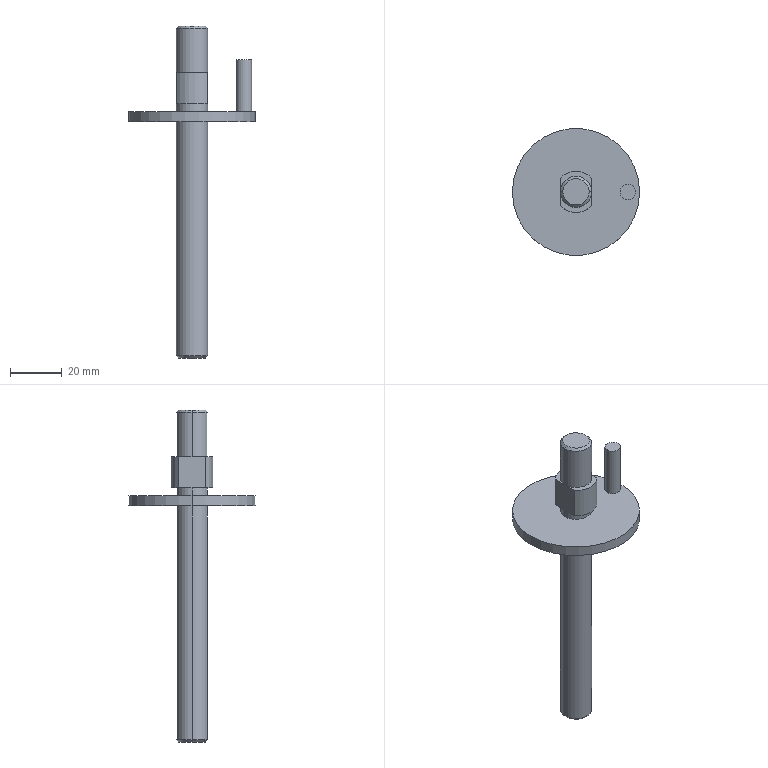Part | SolidWorks | features ICE 5, Chamfer 1, Extrusion 1 | 1 solid | 27 faces | box 49 x 49 x 128 mm | volume 22811 mm3 | cylinder 12 | plane 11 | cone 4 | commonest cylinder face diameters 12 x6 6 x2 16 x2 49 x2
STEP:
#1=CARTESIAN_POINT('',(23.,0.,115.));
#2=VERTEX_POINT('',#1);
#3=CARTESIAN_POINT('',(17.,0.,115.));
#4=VERTEX_POINT('',#3);
#5=CARTESIAN_POINT('',(20.,0.,115.));
#6=DIRECTION('',(0.,0.,1.));
#7=DIRECTION('',(1.,0.,0.));
#8=AXIS2_PLACEMENT_3D('',#5,#6,#7);
#9=CIRCLE('',#8,3.);
#10=EDGE_CURVE('',#2,#4,#9,.T.);
#11=ORIENTED_EDGE('',*,*,#10,.F.);
#12=CARTESIAN_POINT('',(23.,0.,95.));
#13=VERTEX_POINT('',#12);
#14=CARTESIAN_POINT('',(23.,0.,115.));
#15=DIRECTION('',(0.,0.,-1.));
#16=VECTOR('',#15,1000.);
#17=LINE('',#14,#16);
#18=EDGE_CURVE('',#2,#13,#17,.T.);
#19=ORIENTED_EDGE('',*,*,#18,.T.);
#20=CARTESIAN_POINT('',(17.,0.,95.));
#21=VERTEX_POINT('',#20);
#22=CARTESIAN_POINT('',(20.,0.,95.));
#23=DIRECTION('',(0.,0.,1.));
#24=DIRECTION('',(1.,0.,0.));
#25=AXIS2_PLACEMENT_3D('',#22,#23,#24);
#26=CIRCLE('',#25,3.);
#27=EDGE_CURVE('',#13,#21,#26,.T.);
#28=ORIENTED_EDGE('',*,*,#27,.T.);
#29=CARTESIAN_POINT('',(17.,0.,115.));
#30=DIRECTION('',(0.,0.,-1.));
#31=VECTOR('',#30,1000.);
#32=LINE('',#29,#31);
#33=EDGE_CURVE('',#4,#21,#32,.T.);
#34=ORIENTED_EDGE('',*,*,#33,.F.);
#35=EDGE_LOOP('',(#11,#19,#28,#34));
#36=FACE_OUTER_BOUND('',#35,.T.);
#37=CARTESIAN_POINT('',(20.,0.,115.));
#38=DIRECTION('',(0.,0.,-1.));
#39=DIRECTION('',(-1.,0.,0.));
#40=AXIS2_PLACEMENT_3D('',#37,#38,#39);
#41=CYLINDRICAL_SURFACE('',#40,3.);
#42=ADVANCED_FACE('',(#36),#41,.T.);
#43=CARTESIAN_POINT('',(5.1,0.,128.));
#44=VERTEX_POINT('',#43);
#45=CARTESIAN_POINT('',(-5.1,0.,128.));
#46=VERTEX_POINT('',#45);
#47=CARTESIAN_POINT('',(0.,0.,128.));
#48=DIRECTION('',(0.,0.,1.));
#49=DIRECTION('',(1.,0.,0.));
#50=AXIS2_PLACEMENT_3D('',#47,#48,#49);
#51=CIRCLE('',#50,5.1);
#52=EDGE_CURVE('',#44,#46,#51,.T.);
#53=ORIENTED_EDGE('',*,*,#52,.F.);
#54=CARTESIAN_POINT('',(6.,0.,127.1));
#55=VERTEX_POINT('',#54);
#56=CARTESIAN_POINT('',(5.1,0.,128.));
#57=DIRECTION('',(0.7071,0.,-0.7071));
#58=VECTOR('',#57,1000.);
#59=LINE('',#56,#58);
#60=EDGE_CURVE('',#44,#55,#59,.T.);
#61=ORIENTED_EDGE('',*,*,#60,.T.);
#62=CARTESIAN_POINT('',(-6.,0.,127.1));
#63=VERTEX_POINT('',#62);
#64=CARTESIAN_POINT('',(0.,0.,127.1));
#65=DIRECTION('',(0.,0.,-1.));
#66=DIRECTION('',(1.,0.,0.));
#67=AXIS2_PLACEMENT_3D('',#64,#65,#66);
#68=CIRCLE('',#67,6.);
#69=EDGE_CURVE('',#63,#55,#68,.T.);
#70=ORIENTED_EDGE('',*,*,#69,.F.);
#71=CARTESIAN_POINT('',(-5.1,0.,128.));
#72=DIRECTION('',(-0.7071,0.,-0.7071));
#73=VECTOR('',#72,1000.);
#74=LINE('',#71,#73);
#75=EDGE_CURVE('',#46,#63,#74,.T.);
#76=ORIENTED_EDGE('',*,*,#75,.F.);
#77=EDGE_LOOP('',(#53,#61,#70,#76));
#78=FACE_OUTER_BOUND('',#77,.T.);
#79=CARTESIAN_POINT('',(0.,0.,128.));
#80=DIRECTION('',(0.,0.,-1.));
#81=DIRECTION('',(-1.,0.,0.));
#82=AXIS2_PLACEMENT_3D('',#79,#80,#81);
#83=CONICAL_SURFACE('',#82,5.1,0.7854);
#84=ADVANCED_FACE('',(#78),#83,.T.);
#85=CARTESIAN_POINT('',(-5.1,0.,0.));
#86=VERTEX_POINT('',#85);
#87=CARTESIAN_POINT('',(5.1,0.,0.));
#88=VERTEX_POINT('',#87);
#89=CARTESIAN_POINT('',(0.,0.,0.));
#90=DIRECTION('',(0.,0.,-1.));
#91=DIRECTION('',(1.,0.,0.));
#92=AXIS2_PLACEMENT_3D('',#89,#90,#91);
#93=CIRCLE('',#92,5.1);
#94=EDGE_CURVE('',#86,#88,#93,.T.);
#95=ORIENTED_EDGE('',*,*,#94,.F.);
#96=CARTESIAN_POINT('',(-6.,0.,0.9));
#97=VERTEX_POINT('',#96);
#98=CARTESIAN_POINT('',(-6.,0.,0.9));
#99=DIRECTION('',(-0.7071,0.,0.7071));
#100=VECTOR('',#99,1000.);
#101=LINE('',#98,#100);
#102=EDGE_CURVE('',#86,#97,#101,.T.);
#103=ORIENTED_EDGE('',*,*,#102,.T.);
#104=CARTESIAN_POINT('',(6.,0.,0.9));
#105=VERTEX_POINT('',#104);
#106=CARTESIAN_POINT('',(0.,0.,0.9));
#107=DIRECTION('',(0.,0.,1.));
#108=DIRECTION('',(1.,0.,0.));
#109=AXIS2_PLACEMENT_3D('',#106,#107,#108);
#110=CIRCLE('',#109,6.);
#111=EDGE_CURVE('',#105,#97,#110,.T.);
#112=ORIENTED_EDGE('',*,*,#111,.F.);
#113=CARTESIAN_POINT('',(6.,0.,0.9));
#114=DIRECTION('',(0.7071,0.,0.7071));
#115=VECTOR('',#114,1000.);
#116=LINE('',#113,#115);
#117=EDGE_CURVE('',#88,#105,#116,.T.);
#118=ORIENTED_EDGE('',*,*,#117,.F.);
#119=EDGE_LOOP('',(#95,#103,#112,#118));
#120=FACE_OUTER_BOUND('',#119,.T.);
#121=CARTESIAN_POINT('',(0.,0.,0.9));
#122=DIRECTION('',(0.,0.,1.));
#123=DIRECTION('',(1.,0.,0.));
#124=AXIS2_PLACEMENT_3D('',#121,#122,#123);
#125=CONICAL_SURFACE('',#124,6.,0.7854);
#126=ADVANCED_FACE('',(#120),#125,.T.);
#127=ORIENTED_EDGE('',*,*,#69,.T.);
#128=CARTESIAN_POINT('',(6.,0.,110.));
#129=VERTEX_POINT('',#128);
#130=CARTESIAN_POINT('',(6.,0.,128.));
#131=DIRECTION('',(0.,0.,-1.));
#132=VECTOR('',#131,1000.);
#133=LINE('',#130,#132);
#134=EDGE_CURVE('',#55,#129,#133,.T.);
#135=ORIENTED_EDGE('',*,*,#134,.T.);
#136=CARTESIAN_POINT('',(-6.,0.,110.));
#137=VERTEX_POINT('',#136);
#138=CARTESIAN_POINT('',(0.,0.,110.));
#139=DIRECTION('',(0.,0.,1.));
#140=DIRECTION('',(1.,0.,0.));
#141=AXIS2_PLACEMENT_3D('',#138,#139,#140);
#142=CIRCLE('',#141,6.);
#143=EDGE_CURVE('',#129,#137,#142,.T.);
#144=ORIENTED_EDGE('',*,*,#143,.T.);
#145=CARTESIAN_POINT('',(-6.,0.,128.));
#146=DIRECTION('',(0.,0.,-1.));
#147=VECTOR('',#146,1000.);
#148=LINE('',#145,#147);
#149=EDGE_CURVE('',#63,#137,#148,.T.);
#150=ORIENTED_EDGE('',*,*,#149,.F.);
#151=EDGE_LOOP('',(#127,#135,#144,#150));
#152=FACE_OUTER_BOUND('',#151,.T.);
#153=CARTESIAN_POINT('',(0.,0.,128.));
#154=DIRECTION('',(0.,0.,-1.));
#155=DIRECTION('',(-1.,0.,0.));
#156=AXIS2_PLACEMENT_3D('',#153,#154,#155);
#157=CYLINDRICAL_SURFACE('',#156,6.);
#158=ADVANCED_FACE('',(#152),#157,.T.);
#159=CARTESIAN_POINT('',(6.,0.,98.));
#160=VERTEX_POINT('',#159);
#161=CARTESIAN_POINT('',(-6.,0.,98.));
#162=VERTEX_POINT('',#161);
#163=CARTESIAN_POINT('',(0.,0.,98.));
#164=DIRECTION('',(0.,0.,1.));
#165=DIRECTION('',(1.,0.,0.));
#166=AXIS2_PLACEMENT_3D('',#163,#164,#165);
#167=CIRCLE('',#166,6.);
#168=EDGE_CURVE('',#160,#162,#167,.T.);
#169=ORIENTED_EDGE('',*,*,#168,.F.);
#170=CARTESIAN_POINT('',(6.,0.,95.));
#171=VERTEX_POINT('',#170);
#172=CARTESIAN_POINT('',(6.,0.,98.));
#173=DIRECTION('',(0.,0.,-1.));
#174=VECTOR('',#173,1000.);
#175=LINE('',#172,#174);
#176=EDGE_CURVE('',#160,#171,#175,.T.);
#177=ORIENTED_EDGE('',*,*,#176,.T.);
#178=CARTESIAN_POINT('',(-6.,0.,95.));
#179=VERTEX_POINT('',#178);
#180=CARTESIAN_POINT('',(0.,0.,95.));
#181=DIRECTION('',(0.,0.,1.));
#182=DIRECTION('',(1.,0.,0.));
#183=AXIS2_PLACEMENT_3D('',#180,#181,#182);
#184=CIRCLE('',#183,6.);
#185=EDGE_CURVE('',#171,#179,#184,.T.);
#186=ORIENTED_EDGE('',*,*,#185,.T.);
#187=CARTESIAN_POINT('',(-6.,0.,98.));
#188=DIRECTION('',(0.,0.,-1.));
#189=VECTOR('',#188,1000.);
#190=LINE('',#187,#189);
#191=EDGE_CURVE('',#162,#179,#190,.T.);
#192=ORIENTED_EDGE('',*,*,#191,.F.);
#193=EDGE_LOOP('',(#169,#177,#186,#192));
#194=FACE_OUTER_BOUND('',#193,.T.);
#195=CARTESIAN_POINT('',(0.,0.,98.));
#196=DIRECTION('',(0.,0.,-1.));
#197=DIRECTION('',(-1.,0.,0.));
#198=AXIS2_PLACEMENT_3D('',#195,#196,#197);
#199=CYLINDRICAL_SURFACE('',#198,6.);
#200=ADVANCED_FACE('',(#194),#199,.T.);
#201=CARTESIAN_POINT('',(24.5,0.,95.));
#202=VERTEX_POINT('',#201);
#203=CARTESIAN_POINT('',(-24.5,0.,95.));
#204=VERTEX_POINT('',#203);
#205=CARTESIAN_POINT('',(0.,0.,95.));
#206=DIRECTION('',(0.,0.,1.));
#207=DIRECTION('',(1.,0.,0.));
#208=AXIS2_PLACEMENT_3D('',#205,#206,#207);
#209=CIRCLE('',#208,24.5);
#210=EDGE_CURVE('',#202,#204,#209,.T.);
#211=ORIENTED_EDGE('',*,*,#210,.F.);
#212=CARTESIAN_POINT('',(24.5,0.,91.));
#213=VERTEX_POINT('',#212);
#214=CARTESIAN_POINT('',(24.5,0.,95.));
#215=DIRECTION('',(0.,0.,-1.));
#216=VECTOR('',#215,1000.);
#217=LINE('',#214,#216);
#218=EDGE_CURVE('',#202,#213,#217,.T.);
#219=ORIENTED_EDGE('',*,*,#218,.T.);
#220=CARTESIAN_POINT('',(-24.5,0.,91.));
#221=VERTEX_POINT('',#220);
#222=CARTESIAN_POINT('',(0.,0.,91.));
#223=DIRECTION('',(0.,0.,1.));
#224=DIRECTION('',(1.,0.,0.));
#225=AXIS2_PLACEMENT_3D('',#222,#223,#224);
#226=CIRCLE('',#225,24.5);
#227=EDGE_CURVE('',#213,#221,#226,.T.);
#228=ORIENTED_EDGE('',*,*,#227,.T.);
#229=CARTESIAN_POINT('',(-24.5,0.,95.));
#230=DIRECTION('',(0.,0.,-1.));
#231=VECTOR('',#230,1000.);
#232=LINE('',#229,#231);
#233=EDGE_CURVE('',#204,#221,#232,.T.);
#234=ORIENTED_EDGE('',*,*,#233,.F.);
#235=EDGE_LOOP('',(#211,#219,#228,#234));
#236=FACE_OUTER_BOUND('',#235,.T.);
#237=CARTESIAN_POINT('',(0.,0.,95.));
#238=DIRECTION('',(0.,0.,-1.));
#239=DIRECTION('',(-1.,0.,0.));
#240=AXIS2_PLACEMENT_3D('',#237,#238,#239);
#241=CYLINDRICAL_SURFACE('',#240,24.5);
#242=ADVANCED_FACE('',(#236),#241,.T.);
#243=CARTESIAN_POINT('',(6.,0.,91.));
#244=VERTEX_POINT('',#243);
#245=CARTESIAN_POINT('',(-6.,0.,91.));
#246=VERTEX_POINT('',#245);
#247=CARTESIAN_POINT('',(0.,0.,91.));
#248=DIRECTION('',(0.,0.,1.));
#249=DIRECTION('',(1.,0.,0.));
#250=AXIS2_PLACEMENT_3D('',#247,#248,#249);
#251=CIRCLE('',#250,6.);
#252=EDGE_CURVE('',#244,#246,#251,.T.);
#253=ORIENTED_EDGE('',*,*,#252,.F.);
#254=CARTESIAN_POINT('',(6.,0.,91.));
#255=DIRECTION('',(0.,0.,-1.));
#256=VECTOR('',#255,1000.);
#257=LINE('',#254,#256);
#258=EDGE_CURVE('',#244,#105,#257,.T.);
#259=ORIENTED_EDGE('',*,*,#258,.T.);
#260=ORIENTED_EDGE('',*,*,#111,.T.);
#261=CARTESIAN_POINT('',(-6.,0.,91.));
#262=DIRECTION('',(0.,0.,-1.));
#263=VECTOR('',#262,1000.);
#264=LINE('',#261,#263);
#265=EDGE_CURVE('',#246,#97,#264,.T.);
#266=ORIENTED_EDGE('',*,*,#265,.F.);
#267=EDGE_LOOP('',(#253,#259,#260,#266));
#268=FACE_OUTER_BOUND('',#267,.T.);
#269=CARTESIAN_POINT('',(0.,0.,91.));
#270=DIRECTION('',(0.,0.,-1.));
#271=DIRECTION('',(-1.,0.,0.));
#272=AXIS2_PLACEMENT_3D('',#269,#270,#271);
#273=CYLINDRICAL_SURFACE('',#272,6.);
#274=ADVANCED_FACE('',(#268),#273,.T.);
#275=CARTESIAN_POINT('',(0.,0.,95.));
#276=DIRECTION('',(0.,0.,1.));
#277=DIRECTION('',(1.,0.,0.));
#278=AXIS2_PLACEMENT_3D('',#275,#276,#277);
#279=CIRCLE('',#278,6.);
#280=EDGE_CURVE('',#179,#171,#279,.T.);
#281=ORIENTED_EDGE('',*,*,#280,.F.);
#282=ORIENTED_EDGE('',*,*,#185,.F.);
#283=EDGE_LOOP('',(#281,#282));
#284=FACE_BOUND('',#283,.T.);
#285=CARTESIAN_POINT('',(0.,0.,95.));
#286=DIRECTION('',(0.,0.,1.));
#287=DIRECTION('',(1.,0.,0.));
#288=AXIS2_PLACEMENT_3D('',#285,#286,#287);
#289=CIRCLE('',#288,24.5);
#290=EDGE_CURVE('',#204,#202,#289,.T.);
#291=ORIENTED_EDGE('',*,*,#290,.T.);
#292=ORIENTED_EDGE('',*,*,#210,.T.);
#293=EDGE_LOOP('',(#291,#292));
#294=FACE_OUTER_BOUND('',#293,.T.);
#295=CARTESIAN_POINT('',(20.,0.,95.));
#296=DIRECTION('',(0.,0.,1.));
#297=DIRECTION('',(1.,0.,0.));
#298=AXIS2_PLACEMENT_3D('',#295,#296,#297);
#299=CIRCLE('',#298,3.);
#300=EDGE_CURVE('',#21,#13,#299,.T.);
#301=ORIENTED_EDGE('',*,*,#300,.F.);
#302=ORIENTED_EDGE('',*,*,#27,.F.);
#303=EDGE_LOOP('',(#301,#302));
#304=FACE_BOUND('',#303,.T.);
#305=CARTESIAN_POINT('',(0.,0.,95.));
#306=DIRECTION('',(0.,0.,1.));
#307=DIRECTION('',(1.,0.,0.));
#308=AXIS2_PLACEMENT_3D('',#305,#306,#307);
#309=PLANE('',#308);
#310=ADVANCED_FACE('',(#284,#294,#304),#309,.T.);
#311=ORIENTED_EDGE('',*,*,#143,.F.);
#312=CARTESIAN_POINT('',(6.,5.292,110.));
#313=VERTEX_POINT('',#312);
#314=CARTESIAN_POINT('',(6.,5.292,110.));
#315=DIRECTION('',(0.,1.,0.));
#316=VECTOR('',#315,1000.);
#317=LINE('',#314,#316);
#318=EDGE_CURVE('',#129,#313,#317,.T.);
#319=ORIENTED_EDGE('',*,*,#318,.T.);
#320=CARTESIAN_POINT('',(-6.,5.292,110.));
#321=VERTEX_POINT('',#320);
#322=CARTESIAN_POINT('',(0.,0.,110.));
#323=DIRECTION('',(0.,0.,1.));
#324=DIRECTION('',(1.,0.,0.));
#325=AXIS2_PLACEMENT_3D('',#322,#323,#324);
#326=CIRCLE('',#325,8.);
#327=EDGE_CURVE('',#313,#321,#326,.T.);
#328=ORIENTED_EDGE('',*,*,#327,.T.);
#329=CARTESIAN_POINT('',(-6.,5.292,110.));
#330=DIRECTION('',(0.,-1.,0.));
#331=VECTOR('',#330,1000.);
#332=LINE('',#329,#331);
#333=EDGE_CURVE('',#321,#137,#332,.T.);
#334=ORIENTED_EDGE('',*,*,#333,.T.);
#335=EDGE_LOOP('',(#311,#319,#328,#334));
#336=FACE_OUTER_BOUND('',#335,.T.);
#337=CARTESIAN_POINT('',(0.,0.,110.));
#338=DIRECTION('',(0.,0.,1.));
#339=DIRECTION('',(1.,0.,0.));
#340=AXIS2_PLACEMENT_3D('',#337,#338,#339);
#341=PLANE('',#340);
#342=ADVANCED_FACE('',(#336),#341,.T.);
#343=ORIENTED_EDGE('',*,*,#258,.F.);
#344=CARTESIAN_POINT('',(0.,0.,91.));
#345=DIRECTION('',(0.,0.,1.));
#346=DIRECTION('',(1.,0.,0.));
#347=AXIS2_PLACEMENT_3D('',#344,#345,#346);
#348=CIRCLE('',#347,6.);
#349=EDGE_CURVE('',#246,#244,#348,.T.);
#350=ORIENTED_EDGE('',*,*,#349,.F.);
#351=ORIENTED_EDGE('',*,*,#265,.T.);
#352=CARTESIAN_POINT('',(0.,0.,0.9));
#353=DIRECTION('',(0.,0.,1.));
#354=DIRECTION('',(1.,0.,0.));
#355=AXIS2_PLACEMENT_3D('',#352,#353,#354);
#356=CIRCLE('',#355,6.);
#357=EDGE_CURVE('',#97,#105,#356,.T.);
#358=ORIENTED_EDGE('',*,*,#357,.T.);
#359=EDGE_LOOP('',(#343,#350,#351,#358));
#360=FACE_OUTER_BOUND('',#359,.T.);
#361=CARTESIAN_POINT('',(0.,0.,91.));
#362=DIRECTION('',(0.,0.,-1.));
#363=DIRECTION('',(-1.,0.,0.));
#364=AXIS2_PLACEMENT_3D('',#361,#362,#363);
#365=CYLINDRICAL_SURFACE('',#364,6.);
#366=ADVANCED_FACE('',(#360),#365,.T.);
#367=CARTESIAN_POINT('',(0.,0.,0.));
#368=DIRECTION('',(0.,0.,-1.));
#369=DIRECTION('',(1.,0.,0.));
#370=AXIS2_PLACEMENT_3D('',#367,#368,#369);
#371=CIRCLE('',#370,5.1);
#372=EDGE_CURVE('',#88,#86,#371,.T.);
#373=ORIENTED_EDGE('',*,*,#372,.T.);
#374=ORIENTED_EDGE('',*,*,#94,.T.);
#375=EDGE_LOOP('',(#373,#374));
#376=FACE_OUTER_BOUND('',#375,.T.);
#377=CARTESIAN_POINT('',(0.,0.,0.));
#378=DIRECTION('',(0.,0.,1.));
#379=DIRECTION('',(1.,0.,0.));
#380=AXIS2_PLACEMENT_3D('',#377,#378,#379);
#381=PLANE('',#380);
#382=ADVANCED_FACE('',(#376),#381,.F.);
#383=CARTESIAN_POINT('',(0.,0.,91.));
#384=DIRECTION('',(0.,0.,1.));
#385=DIRECTION('',(1.,0.,0.));
#386=AXIS2_PLACEMENT_3D('',#383,#384,#385);
#387=CIRCLE('',#386,24.5);
#388=EDGE_CURVE('',#221,#213,#387,.T.);
#389=ORIENTED_EDGE('',*,*,#388,.F.);
#390=ORIENTED_EDGE('',*,*,#227,.F.);
#391=EDGE_LOOP('',(#389,#390));
#392=FACE_OUTER_BOUND('',#391,.T.);
#393=ORIENTED_EDGE('',*,*,#349,.T.);
#394=ORIENTED_EDGE('',*,*,#252,.T.);
#395=EDGE_LOOP('',(#393,#394));
#396=FACE_BOUND('',#395,.T.);
#397=CARTESIAN_POINT('',(0.,0.,91.));
#398=DIRECTION('',(0.,0.,1.));
#399=DIRECTION('',(1.,0.,0.));
#400=AXIS2_PLACEMENT_3D('',#397,#398,#399);
#401=PLANE('',#400);
#402=ADVANCED_FACE('',(#392,#396),#401,.F.);
#403=ORIENTED_EDGE('',*,*,#218,.F.);
#404=ORIENTED_EDGE('',*,*,#290,.F.);
#405=ORIENTED_EDGE('',*,*,#233,.T.);
#406=ORIENTED_EDGE('',*,*,#388,.T.);
#407=EDGE_LOOP('',(#403,#404,#405,#406));
#408=FACE_OUTER_BOUND('',#407,.T.);
#409=CARTESIAN_POINT('',(0.,0.,95.));
#410=DIRECTION('',(0.,0.,-1.));
#411=DIRECTION('',(-1.,0.,0.));
#412=AXIS2_PLACEMENT_3D('',#409,#410,#411);
#413=CYLINDRICAL_SURFACE('',#412,24.5);
#414=ADVANCED_FACE('',(#408),#413,.T.);
#415=ORIENTED_EDGE('',*,*,#176,.F.);
#416=CARTESIAN_POINT('',(0.,0.,98.));
#417=DIRECTION('',(0.,0.,1.));
#418=DIRECTION('',(1.,0.,0.));
#419=AXIS2_PLACEMENT_3D('',#416,#417,#418);
#420=CIRCLE('',#419,6.);
#421=EDGE_CURVE('',#162,#160,#420,.T.);
#422=ORIENTED_EDGE('',*,*,#421,.F.);
#423=ORIENTED_EDGE('',*,*,#191,.T.);
#424=ORIENTED_EDGE('',*,*,#280,.T.);
#425=EDGE_LOOP('',(#415,#422,#423,#424));
#426=FACE_OUTER_BOUND('',#425,.T.);
#427=CARTESIAN_POINT('',(0.,0.,98.));
#428=DIRECTION('',(0.,0.,-1.));
#429=DIRECTION('',(-1.,0.,0.));
#430=AXIS2_PLACEMENT_3D('',#427,#428,#429);
#431=CYLINDRICAL_SURFACE('',#430,6.);
#432=ADVANCED_FACE('',(#426),#431,.T.);
#433=CARTESIAN_POINT('',(6.,5.292,98.));
#434=VERTEX_POINT('',#433);
#435=CARTESIAN_POINT('',(6.,5.292,98.));
#436=DIRECTION('',(0.,1.,0.));
#437=VECTOR('',#436,1000.);
#438=LINE('',#435,#437);
#439=EDGE_CURVE('',#160,#434,#438,.T.);
#440=ORIENTED_EDGE('',*,*,#439,.F.);
#441=ORIENTED_EDGE('',*,*,#168,.T.);
#442=CARTESIAN_POINT('',(-6.,5.292,98.));
#443=VERTEX_POINT('',#442);
#444=CARTESIAN_POINT('',(-6.,5.292,98.));
#445=DIRECTION('',(0.,-1.,0.));
#446=VECTOR('',#445,1000.);
#447=LINE('',#444,#446);
#448=EDGE_CURVE('',#443,#162,#447,.T.);
#449=ORIENTED_EDGE('',*,*,#448,.F.);
#450=CARTESIAN_POINT('',(0.,0.,98.));
#451=DIRECTION('',(0.,0.,1.));
#452=DIRECTION('',(1.,0.,0.));
#453=AXIS2_PLACEMENT_3D('',#450,#451,#452);
#454=CIRCLE('',#453,8.);
#455=EDGE_CURVE('',#434,#443,#454,.T.);
#456=ORIENTED_EDGE('',*,*,#455,.F.);
#457=EDGE_LOOP('',(#440,#441,#449,#456));
#458=FACE_OUTER_BOUND('',#457,.T.);
#459=CARTESIAN_POINT('',(0.,0.,98.));
#460=DIRECTION('',(0.,0.,1.));
#461=DIRECTION('',(1.,0.,0.));
#462=AXIS2_PLACEMENT_3D('',#459,#460,#461);
#463=PLANE('',#462);
#464=ADVANCED_FACE('',(#458),#463,.F.);
#465=CARTESIAN_POINT('',(-6.,-5.292,98.));
#466=VERTEX_POINT('',#465);
#467=CARTESIAN_POINT('',(-6.,5.292,98.));
#468=DIRECTION('',(0.,-1.,0.));
#469=VECTOR('',#468,1000.);
#470=LINE('',#467,#469);
#471=EDGE_CURVE('',#162,#466,#470,.T.);
#472=ORIENTED_EDGE('',*,*,#471,.F.);
#473=ORIENTED_EDGE('',*,*,#421,.T.);
#474=CARTESIAN_POINT('',(6.,-5.292,98.));
#475=VERTEX_POINT('',#474);
#476=CARTESIAN_POINT('',(6.,5.292,98.));
#477=DIRECTION('',(0.,1.,0.));
#478=VECTOR('',#477,1000.);
#479=LINE('',#476,#478);
#480=EDGE_CURVE('',#475,#160,#479,.T.);
#481=ORIENTED_EDGE('',*,*,#480,.F.);
#482=CARTESIAN_POINT('',(0.,0.,98.));
#483=DIRECTION('',(0.,0.,1.));
#484=DIRECTION('',(1.,0.,0.));
#485=AXIS2_PLACEMENT_3D('',#482,#483,#484);
#486=CIRCLE('',#485,8.);
#487=EDGE_CURVE('',#466,#475,#486,.T.);
#488=ORIENTED_EDGE('',*,*,#487,.F.);
#489=EDGE_LOOP('',(#472,#473,#481,#488));
#490=FACE_OUTER_BOUND('',#489,.T.);
#491=CARTESIAN_POINT('',(0.,0.,98.));
#492=DIRECTION('',(0.,0.,1.));
#493=DIRECTION('',(1.,0.,0.));
#494=AXIS2_PLACEMENT_3D('',#491,#492,#493);
#495=PLANE('',#494);
#496=ADVANCED_FACE('',(#490),#495,.F.);
#497=ORIENTED_EDGE('',*,*,#455,.T.);
#498=CARTESIAN_POINT('',(-6.,5.292,110.));
#499=DIRECTION('',(0.,0.,-1.));
#500=VECTOR('',#499,1000.);
#501=LINE('',#498,#500);
#502=EDGE_CURVE('',#321,#443,#501,.T.);
#503=ORIENTED_EDGE('',*,*,#502,.F.);
#504=ORIENTED_EDGE('',*,*,#327,.F.);
#505=CARTESIAN_POINT('',(6.,5.292,110.));
#506=DIRECTION('',(0.,0.,-1.));
#507=VECTOR('',#506,1000.);
#508=LINE('',#505,#507);
#509=EDGE_CURVE('',#313,#434,#508,.T.);
#510=ORIENTED_EDGE('',*,*,#509,.T.);
#511=EDGE_LOOP('',(#497,#503,#504,#510));
#512=FACE_OUTER_BOUND('',#511,.T.);
#513=CARTESIAN_POINT('',(0.,0.,110.));
#514=DIRECTION('',(0.,0.,-1.));
#515=DIRECTION('',(-1.,0.,0.));
#516=AXIS2_PLACEMENT_3D('',#513,#514,#515);
#517=CYLINDRICAL_SURFACE('',#516,8.);
#518=ADVANCED_FACE('',(#512),#517,.T.);
#519=ORIENTED_EDGE('',*,*,#448,.T.);
#520=ORIENTED_EDGE('',*,*,#471,.T.);
#521=CARTESIAN_POINT('',(-6.,-5.292,110.));
#522=VERTEX_POINT('',#521);
#523=CARTESIAN_POINT('',(-6.,-5.292,110.));
#524=DIRECTION('',(0.,0.,-1.));
#525=VECTOR('',#524,1000.);
#526=LINE('',#523,#525);
#527=EDGE_CURVE('',#522,#466,#526,.T.);
#528=ORIENTED_EDGE('',*,*,#527,.F.);
#529=CARTESIAN_POINT('',(-6.,5.292,110.));
#530=DIRECTION('',(0.,-1.,0.));
#531=VECTOR('',#530,1000.);
#532=LINE('',#529,#531);
#533=EDGE_CURVE('',#137,#522,#532,.T.);
#534=ORIENTED_EDGE('',*,*,#533,.F.);
#535=ORIENTED_EDGE('',*,*,#333,.F.);
#536=ORIENTED_EDGE('',*,*,#502,.T.);
#537=EDGE_LOOP('',(#519,#520,#528,#534,#535,#536));
#538=FACE_OUTER_BOUND('',#537,.T.);
#539=CARTESIAN_POINT('',(-6.,5.292,110.));
#540=DIRECTION('',(1.,0.,0.));
#541=DIRECTION('',(0.,0.,-1.));
#542=AXIS2_PLACEMENT_3D('',#539,#540,#541);
#543=PLANE('',#542);
#544=ADVANCED_FACE('',(#538),#543,.F.);
#545=ORIENTED_EDGE('',*,*,#487,.T.);
#546=CARTESIAN_POINT('',(6.,-5.292,110.));
#547=VERTEX_POINT('',#546);
#548=CARTESIAN_POINT('',(6.,-5.292,110.));
#549=DIRECTION('',(0.,0.,-1.));
#550=VECTOR('',#549,1000.);
#551=LINE('',#548,#550);
#552=EDGE_CURVE('',#547,#475,#551,.T.);
#553=ORIENTED_EDGE('',*,*,#552,.F.);
#554=CARTESIAN_POINT('',(0.,0.,110.));
#555=DIRECTION('',(0.,0.,1.));
#556=DIRECTION('',(1.,0.,0.));
#557=AXIS2_PLACEMENT_3D('',#554,#555,#556);
#558=CIRCLE('',#557,8.);
#559=EDGE_CURVE('',#522,#547,#558,.T.);
#560=ORIENTED_EDGE('',*,*,#559,.F.);
#561=ORIENTED_EDGE('',*,*,#527,.T.);
#562=EDGE_LOOP('',(#545,#553,#560,#561));
#563=FACE_OUTER_BOUND('',#562,.T.);
#564=CARTESIAN_POINT('',(0.,0.,110.));
#565=DIRECTION('',(0.,0.,-1.));
#566=DIRECTION('',(-1.,0.,0.));
#567=AXIS2_PLACEMENT_3D('',#564,#565,#566);
#568=CYLINDRICAL_SURFACE('',#567,8.);
#569=ADVANCED_FACE('',(#563),#568,.T.);
#570=ORIENTED_EDGE('',*,*,#480,.T.);
#571=ORIENTED_EDGE('',*,*,#439,.T.);
#572=ORIENTED_EDGE('',*,*,#509,.F.);
#573=ORIENTED_EDGE('',*,*,#318,.F.);
#574=CARTESIAN_POINT('',(6.,5.292,110.));
#575=DIRECTION('',(0.,1.,0.));
#576=VECTOR('',#575,1000.);
#577=LINE('',#574,#576);
#578=EDGE_CURVE('',#547,#129,#577,.T.);
#579=ORIENTED_EDGE('',*,*,#578,.F.);
#580=ORIENTED_EDGE('',*,*,#552,.T.);
#581=EDGE_LOOP('',(#570,#571,#572,#573,#579,#580));
#582=FACE_OUTER_BOUND('',#581,.T.);
#583=CARTESIAN_POINT('',(6.,5.292,110.));
#584=DIRECTION('',(-1.,0.,0.));
#585=DIRECTION('',(0.,-1.,0.));
#586=AXIS2_PLACEMENT_3D('',#583,#584,#585);
#587=PLANE('',#586);
#588=ADVANCED_FACE('',(#582),#587,.F.);
#589=CARTESIAN_POINT('',(0.,0.,110.));
#590=DIRECTION('',(0.,0.,1.));
#591=DIRECTION('',(1.,0.,0.));
#592=AXIS2_PLACEMENT_3D('',#589,#590,#591);
#593=CIRCLE('',#592,6.);
#594=EDGE_CURVE('',#137,#129,#593,.T.);
#595=ORIENTED_EDGE('',*,*,#594,.F.);
#596=ORIENTED_EDGE('',*,*,#533,.T.);
#597=ORIENTED_EDGE('',*,*,#559,.T.);
#598=ORIENTED_EDGE('',*,*,#578,.T.);
#599=EDGE_LOOP('',(#595,#596,#597,#598));
#600=FACE_OUTER_BOUND('',#599,.T.);
#601=CARTESIAN_POINT('',(0.,0.,110.));
#602=DIRECTION('',(0.,0.,1.));
#603=DIRECTION('',(1.,0.,0.));
#604=AXIS2_PLACEMENT_3D('',#601,#602,#603);
#605=PLANE('',#604);
#606=ADVANCED_FACE('',(#600),#605,.T.);
#607=ORIENTED_EDGE('',*,*,#134,.F.);
#608=CARTESIAN_POINT('',(0.,0.,127.1));
#609=DIRECTION('',(0.,0.,-1.));
#610=DIRECTION('',(1.,0.,0.));
#611=AXIS2_PLACEMENT_3D('',#608,#609,#610);
#612=CIRCLE('',#611,6.);
#613=EDGE_CURVE('',#55,#63,#612,.T.);
#614=ORIENTED_EDGE('',*,*,#613,.T.);
#615=ORIENTED_EDGE('',*,*,#149,.T.);
#616=ORIENTED_EDGE('',*,*,#594,.T.);
#617=EDGE_LOOP('',(#607,#614,#615,#616));
#618=FACE_OUTER_BOUND('',#617,.T.);
#619=CARTESIAN_POINT('',(0.,0.,128.));
#620=DIRECTION('',(0.,0.,-1.));
#621=DIRECTION('',(-1.,0.,0.));
#622=AXIS2_PLACEMENT_3D('',#619,#620,#621);
#623=CYLINDRICAL_SURFACE('',#622,6.);
#624=ADVANCED_FACE('',(#618),#623,.T.);
#625=CARTESIAN_POINT('',(0.,0.,128.));
#626=DIRECTION('',(0.,0.,1.));
#627=DIRECTION('',(1.,0.,0.));
#628=AXIS2_PLACEMENT_3D('',#625,#626,#627);
#629=CIRCLE('',#628,5.1);
#630=EDGE_CURVE('',#46,#44,#629,.T.);
#631=ORIENTED_EDGE('',*,*,#630,.T.);
#632=ORIENTED_EDGE('',*,*,#52,.T.);
#633=EDGE_LOOP('',(#631,#632));
#634=FACE_OUTER_BOUND('',#633,.T.);
#635=CARTESIAN_POINT('',(0.,0.,128.));
#636=DIRECTION('',(0.,0.,1.));
#637=DIRECTION('',(1.,0.,0.));
#638=AXIS2_PLACEMENT_3D('',#635,#636,#637);
#639=PLANE('',#638);
#640=ADVANCED_FACE('',(#634),#639,.T.);
#641=ORIENTED_EDGE('',*,*,#102,.F.);
#642=ORIENTED_EDGE('',*,*,#372,.F.);
#643=ORIENTED_EDGE('',*,*,#117,.T.);
#644=ORIENTED_EDGE('',*,*,#357,.F.);
#645=EDGE_LOOP('',(#641,#642,#643,#644));
#646=FACE_OUTER_BOUND('',#645,.T.);
#647=CARTESIAN_POINT('',(0.,0.,0.9));
#648=DIRECTION('',(0.,0.,1.));
#649=DIRECTION('',(1.,0.,0.));
#650=AXIS2_PLACEMENT_3D('',#647,#648,#649);
#651=CONICAL_SURFACE('',#650,6.,0.7854);
#652=ADVANCED_FACE('',(#646),#651,.T.);
#653=ORIENTED_EDGE('',*,*,#60,.F.);
#654=ORIENTED_EDGE('',*,*,#630,.F.);
#655=ORIENTED_EDGE('',*,*,#75,.T.);
#656=ORIENTED_EDGE('',*,*,#613,.F.);
#657=EDGE_LOOP('',(#653,#654,#655,#656));
#658=FACE_OUTER_BOUND('',#657,.T.);
#659=CARTESIAN_POINT('',(0.,0.,128.));
#660=DIRECTION('',(0.,0.,-1.));
#661=DIRECTION('',(-1.,0.,0.));
#662=AXIS2_PLACEMENT_3D('',#659,#660,#661);
#663=CONICAL_SURFACE('',#662,5.1,0.7854);
#664=ADVANCED_FACE('',(#658),#663,.T.);
#665=ORIENTED_EDGE('',*,*,#18,.F.);
#666=CARTESIAN_POINT('',(20.,0.,115.));
#667=DIRECTION('',(0.,0.,1.));
#668=DIRECTION('',(1.,0.,0.));
#669=AXIS2_PLACEMENT_3D('',#666,#667,#668);
#670=CIRCLE('',#669,3.);
#671=EDGE_CURVE('',#4,#2,#670,.T.);
#672=ORIENTED_EDGE('',*,*,#671,.F.);
#673=ORIENTED_EDGE('',*,*,#33,.T.);
#674=ORIENTED_EDGE('',*,*,#300,.T.);
#675=EDGE_LOOP('',(#665,#672,#673,#674));
#676=FACE_OUTER_BOUND('',#675,.T.);
#677=CARTESIAN_POINT('',(20.,0.,115.));
#678=DIRECTION('',(0.,0.,-1.));
#679=DIRECTION('',(-1.,0.,0.));
#680=AXIS2_PLACEMENT_3D('',#677,#678,#679);
#681=CYLINDRICAL_SURFACE('',#680,3.);
#682=ADVANCED_FACE('',(#676),#681,.T.);
#683=ORIENTED_EDGE('',*,*,#671,.T.);
#684=ORIENTED_EDGE('',*,*,#10,.T.);
#685=EDGE_LOOP('',(#683,#684));
#686=FACE_OUTER_BOUND('',#685,.T.);
#687=CARTESIAN_POINT('',(20.,0.,115.));
#688=DIRECTION('',(0.,0.,1.));
#689=DIRECTION('',(1.,0.,0.));
#690=AXIS2_PLACEMENT_3D('',#687,#688,#689);
#691=PLANE('',#690);
#692=ADVANCED_FACE('',(#686),#691,.T.);
#693=CLOSED_SHELL('',(#42,#84,#126,#158,#200,#242,#274,#310,#342,#366,#382,#402,#414,#432,#464,#496,#518,#544,#569,#588,#606,#624,#640,#652,#664,#682,#692));
#694=MANIFOLD_SOLID_BREP('',#693);
#695=CARTESIAN_POINT('',(0.,0.,0.));
#696=DIRECTION('',(0.,0.,1.));
#697=DIRECTION('',(1.,0.,0.));
#698=AXIS2_PLACEMENT_3D('',#695,#696,#697);
#699=(LENGTH_UNIT()NAMED_UNIT(*)SI_UNIT(.MILLI.,.METRE.));
#700=UNCERTAINTY_MEASURE_WITH_UNIT(LENGTH_MEASURE(0.00001),#699,'','');
#701=(NAMED_UNIT(*)PLANE_ANGLE_UNIT()SI_UNIT($,.RADIAN.));
#702=(NAMED_UNIT(*)SI_UNIT($,.STERADIAN.)SOLID_ANGLE_UNIT());
#703=(GEOMETRIC_REPRESENTATION_CONTEXT(3)GLOBAL_UNCERTAINTY_ASSIGNED_CONTEXT((#700))GLOBAL_UNIT_ASSIGNED_CONTEXT((#699,#701,#702))REPRESENTATION_CONTEXT('',''));
#704=ADVANCED_BREP_SHAPE_REPRESENTATION('',(#694,#698),#703);